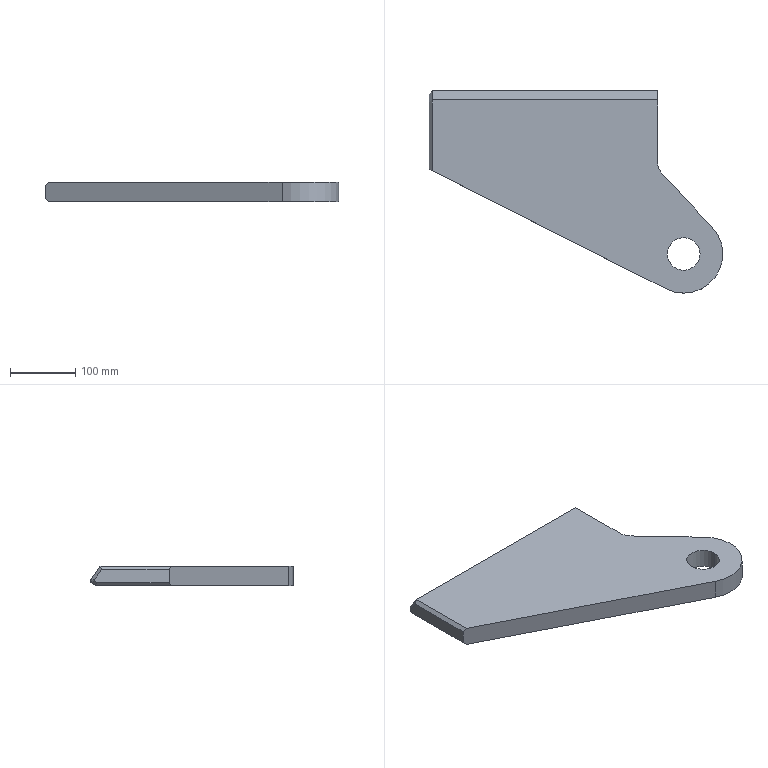Part | SolidWorks | features ICE 2, Chamfer 1, Extrusion 1, Fillet 1 | 1 solid | 18 faces | box 450 x 310 x 30 mm | volume 2452463 mm3 | plane 14 | cylinder 4 | commonest cylinder face diameters 50 x2 60 x1 120 x1
STEP:
#1=CARTESIAN_POINT('',(-25.,0.,30.));
#2=VERTEX_POINT('',#1);
#3=CARTESIAN_POINT('',(25.,0.,30.));
#4=VERTEX_POINT('',#3);
#5=CARTESIAN_POINT('',(0.,0.,30.));
#6=DIRECTION('',(0.,0.,1.));
#7=DIRECTION('',(1.,0.,0.));
#8=AXIS2_PLACEMENT_3D('',#5,#6,#7);
#9=CIRCLE('',#8,25.);
#10=EDGE_CURVE('',#2,#4,#9,.T.);
#11=ORIENTED_EDGE('',*,*,#10,.T.);
#12=CARTESIAN_POINT('',(25.,0.,0.));
#13=VERTEX_POINT('',#12);
#14=CARTESIAN_POINT('',(25.,0.,30.));
#15=DIRECTION('',(0.,0.,-1.));
#16=VECTOR('',#15,1000.);
#17=LINE('',#14,#16);
#18=EDGE_CURVE('',#4,#13,#17,.T.);
#19=ORIENTED_EDGE('',*,*,#18,.T.);
#20=CARTESIAN_POINT('',(-25.,0.,0.));
#21=VERTEX_POINT('',#20);
#22=CARTESIAN_POINT('',(0.,0.,0.));
#23=DIRECTION('',(0.,0.,1.));
#24=DIRECTION('',(1.,0.,0.));
#25=AXIS2_PLACEMENT_3D('',#22,#23,#24);
#26=CIRCLE('',#25,25.);
#27=EDGE_CURVE('',#21,#13,#26,.T.);
#28=ORIENTED_EDGE('',*,*,#27,.F.);
#29=CARTESIAN_POINT('',(-25.,0.,30.));
#30=DIRECTION('',(0.,0.,-1.));
#31=VECTOR('',#30,1000.);
#32=LINE('',#29,#31);
#33=EDGE_CURVE('',#2,#21,#32,.T.);
#34=ORIENTED_EDGE('',*,*,#33,.F.);
#35=EDGE_LOOP('',(#11,#19,#28,#34));
#36=FACE_OUTER_BOUND('',#35,.T.);
#37=CARTESIAN_POINT('',(0.,0.,30.));
#38=DIRECTION('',(0.,0.,-1.));
#39=DIRECTION('',(-1.,0.,0.));
#40=AXIS2_PLACEMENT_3D('',#37,#38,#39);
#41=CYLINDRICAL_SURFACE('',#40,25.);
#42=ADVANCED_FACE('',(#36),#41,.F.);
#43=CARTESIAN_POINT('',(-385.,235.996,30.));
#44=VERTEX_POINT('',#43);
#45=CARTESIAN_POINT('',(-40.,235.996,30.));
#46=VERTEX_POINT('',#45);
#47=CARTESIAN_POINT('',(-390.,235.996,30.));
#48=DIRECTION('',(1.,0.,0.));
#49=VECTOR('',#48,1000.);
#50=LINE('',#47,#49);
#51=EDGE_CURVE('',#44,#46,#50,.T.);
#52=ORIENTED_EDGE('',*,*,#51,.F.);
#53=CARTESIAN_POINT('',(-385.,127.471,30.));
#54=VERTEX_POINT('',#53);
#55=CARTESIAN_POINT('',(-385.,130.,30.));
#56=DIRECTION('',(0.,-1.,0.));
#57=VECTOR('',#56,1000.);
#58=LINE('',#55,#57);
#59=EDGE_CURVE('',#44,#54,#58,.T.);
#60=ORIENTED_EDGE('',*,*,#59,.T.);
#61=CARTESIAN_POINT('',(-27.078,-53.542,30.));
#62=VERTEX_POINT('',#61);
#63=CARTESIAN_POINT('',(-390.,130.,30.));
#64=DIRECTION('',(0.8924,-0.4513,0.));
#65=VECTOR('',#64,1000.);
#66=LINE('',#63,#65);
#67=EDGE_CURVE('',#54,#62,#66,.T.);
#68=ORIENTED_EDGE('',*,*,#67,.T.);
#69=CARTESIAN_POINT('',(43.682,41.133,30.));
#70=VERTEX_POINT('',#69);
#71=CARTESIAN_POINT('',(0.,0.,30.));
#72=DIRECTION('',(0.,0.,1.));
#73=DIRECTION('',(1.,0.,0.));
#74=AXIS2_PLACEMENT_3D('',#71,#72,#73);
#75=CIRCLE('',#74,60.);
#76=EDGE_CURVE('',#62,#70,#75,.T.);
#77=ORIENTED_EDGE('',*,*,#76,.T.);
#78=CARTESIAN_POINT('',(-31.841,121.335,30.));
#79=VERTEX_POINT('',#78);
#80=CARTESIAN_POINT('',(-40.,130.,30.));
#81=DIRECTION('',(-0.6855,0.728,0.));
#82=VECTOR('',#81,1000.);
#83=LINE('',#80,#82);
#84=EDGE_CURVE('',#70,#79,#83,.T.);
#85=ORIENTED_EDGE('',*,*,#84,.T.);
#86=CARTESIAN_POINT('',(-40.,141.902,30.));
#87=VERTEX_POINT('',#86);
#88=CARTESIAN_POINT('',(-10.,141.902,30.));
#89=DIRECTION('',(0.,0.,-1.));
#90=DIRECTION('',(1.,0.,0.));
#91=AXIS2_PLACEMENT_3D('',#88,#89,#90);
#92=CIRCLE('',#91,30.);
#93=EDGE_CURVE('',#79,#87,#92,.T.);
#94=ORIENTED_EDGE('',*,*,#93,.T.);
#95=CARTESIAN_POINT('',(-40.,250.,30.));
#96=DIRECTION('',(0.,1.,0.));
#97=VECTOR('',#96,1000.);
#98=LINE('',#95,#97);
#99=EDGE_CURVE('',#87,#46,#98,.T.);
#100=ORIENTED_EDGE('',*,*,#99,.T.);
#101=EDGE_LOOP('',(#52,#60,#68,#77,#85,#94,#100));
#102=FACE_OUTER_BOUND('',#101,.T.);
#103=ORIENTED_EDGE('',*,*,#10,.F.);
#104=CARTESIAN_POINT('',(0.,0.,30.));
#105=DIRECTION('',(0.,0.,1.));
#106=DIRECTION('',(1.,0.,0.));
#107=AXIS2_PLACEMENT_3D('',#104,#105,#106);
#108=CIRCLE('',#107,25.);
#109=EDGE_CURVE('',#4,#2,#108,.T.);
#110=ORIENTED_EDGE('',*,*,#109,.F.);
#111=EDGE_LOOP('',(#103,#110));
#112=FACE_BOUND('',#111,.T.);
#113=CARTESIAN_POINT('',(0.,0.,30.));
#114=DIRECTION('',(0.,0.,1.));
#115=DIRECTION('',(1.,0.,0.));
#116=AXIS2_PLACEMENT_3D('',#113,#114,#115);
#117=PLANE('',#116);
#118=ADVANCED_FACE('',(#102,#112),#117,.T.);
#119=CARTESIAN_POINT('',(-385.,127.471,0.));
#120=VERTEX_POINT('',#119);
#121=CARTESIAN_POINT('',(-27.078,-53.542,0.));
#122=VERTEX_POINT('',#121);
#123=CARTESIAN_POINT('',(-390.,130.,0.));
#124=DIRECTION('',(0.8924,-0.4513,0.));
#125=VECTOR('',#124,1000.);
#126=LINE('',#123,#125);
#127=EDGE_CURVE('',#120,#122,#126,.T.);
#128=ORIENTED_EDGE('',*,*,#127,.F.);
#129=CARTESIAN_POINT('',(-385.,242.859,0.));
#130=VERTEX_POINT('',#129);
#131=CARTESIAN_POINT('',(-385.,0.,0.));
#132=DIRECTION('',(0.,1.,0.));
#133=VECTOR('',#132,1000.);
#134=LINE('',#131,#133);
#135=EDGE_CURVE('',#120,#130,#134,.T.);
#136=ORIENTED_EDGE('',*,*,#135,.T.);
#137=CARTESIAN_POINT('',(-40.,242.859,0.));
#138=VERTEX_POINT('',#137);
#139=CARTESIAN_POINT('',(-390.,242.859,0.));
#140=DIRECTION('',(1.,0.,0.));
#141=VECTOR('',#140,1000.);
#142=LINE('',#139,#141);
#143=EDGE_CURVE('',#130,#138,#142,.T.);
#144=ORIENTED_EDGE('',*,*,#143,.T.);
#145=CARTESIAN_POINT('',(-40.,141.902,0.));
#146=VERTEX_POINT('',#145);
#147=CARTESIAN_POINT('',(-40.,250.,0.));
#148=DIRECTION('',(0.,1.,0.));
#149=VECTOR('',#148,1000.);
#150=LINE('',#147,#149);
#151=EDGE_CURVE('',#146,#138,#150,.T.);
#152=ORIENTED_EDGE('',*,*,#151,.F.);
#153=CARTESIAN_POINT('',(-31.841,121.335,0.));
#154=VERTEX_POINT('',#153);
#155=CARTESIAN_POINT('',(-10.,141.902,0.));
#156=DIRECTION('',(0.,0.,1.));
#157=DIRECTION('',(1.,0.,0.));
#158=AXIS2_PLACEMENT_3D('',#155,#156,#157);
#159=CIRCLE('',#158,30.);
#160=EDGE_CURVE('',#146,#154,#159,.T.);
#161=ORIENTED_EDGE('',*,*,#160,.T.);
#162=CARTESIAN_POINT('',(43.682,41.133,0.));
#163=VERTEX_POINT('',#162);
#164=CARTESIAN_POINT('',(-40.,130.,0.));
#165=DIRECTION('',(-0.6855,0.728,0.));
#166=VECTOR('',#165,1000.);
#167=LINE('',#164,#166);
#168=EDGE_CURVE('',#163,#154,#167,.T.);
#169=ORIENTED_EDGE('',*,*,#168,.F.);
#170=CARTESIAN_POINT('',(0.,0.,0.));
#171=DIRECTION('',(0.,0.,1.));
#172=DIRECTION('',(1.,0.,0.));
#173=AXIS2_PLACEMENT_3D('',#170,#171,#172);
#174=CIRCLE('',#173,60.);
#175=EDGE_CURVE('',#122,#163,#174,.T.);
#176=ORIENTED_EDGE('',*,*,#175,.F.);
#177=EDGE_LOOP('',(#128,#136,#144,#152,#161,#169,#176));
#178=FACE_OUTER_BOUND('',#177,.T.);
#179=ORIENTED_EDGE('',*,*,#27,.T.);
#180=CARTESIAN_POINT('',(0.,0.,0.));
#181=DIRECTION('',(0.,0.,1.));
#182=DIRECTION('',(1.,0.,0.));
#183=AXIS2_PLACEMENT_3D('',#180,#181,#182);
#184=CIRCLE('',#183,25.);
#185=EDGE_CURVE('',#13,#21,#184,.T.);
#186=ORIENTED_EDGE('',*,*,#185,.T.);
#187=EDGE_LOOP('',(#179,#186));
#188=FACE_BOUND('',#187,.T.);
#189=CARTESIAN_POINT('',(0.,0.,0.));
#190=DIRECTION('',(0.,0.,1.));
#191=DIRECTION('',(1.,0.,0.));
#192=AXIS2_PLACEMENT_3D('',#189,#190,#191);
#193=PLANE('',#192);
#194=ADVANCED_FACE('',(#178,#188),#193,.F.);
#195=ORIENTED_EDGE('',*,*,#99,.F.);
#196=CARTESIAN_POINT('',(-40.,141.902,0.));
#197=DIRECTION('',(0.,0.,-1.));
#198=VECTOR('',#197,1000.);
#199=LINE('',#196,#198);
#200=EDGE_CURVE('',#87,#146,#199,.T.);
#201=ORIENTED_EDGE('',*,*,#200,.T.);
#202=ORIENTED_EDGE('',*,*,#151,.T.);
#203=CARTESIAN_POINT('',(-40.,250.,5.));
#204=VERTEX_POINT('',#203);
#205=CARTESIAN_POINT('',(-40.,261.746,13.225));
#206=DIRECTION('',(0.,0.8192,0.5736));
#207=VECTOR('',#206,1000.);
#208=LINE('',#205,#207);
#209=EDGE_CURVE('',#138,#204,#208,.T.);
#210=ORIENTED_EDGE('',*,*,#209,.T.);
#211=CARTESIAN_POINT('',(-40.,250.,10.));
#212=VERTEX_POINT('',#211);
#213=CARTESIAN_POINT('',(-40.,250.,30.));
#214=DIRECTION('',(0.,0.,-1.));
#215=VECTOR('',#214,1000.);
#216=LINE('',#213,#215);
#217=EDGE_CURVE('',#212,#204,#216,.T.);
#218=ORIENTED_EDGE('',*,*,#217,.F.);
#219=CARTESIAN_POINT('',(-40.,240.603,23.42));
#220=DIRECTION('',(0.,-0.5736,0.8192));
#221=VECTOR('',#220,1000.);
#222=LINE('',#219,#221);
#223=EDGE_CURVE('',#212,#46,#222,.T.);
#224=ORIENTED_EDGE('',*,*,#223,.T.);
#225=EDGE_LOOP('',(#195,#201,#202,#210,#218,#224));
#226=FACE_OUTER_BOUND('',#225,.T.);
#227=CARTESIAN_POINT('',(-40.,250.,30.));
#228=DIRECTION('',(-1.,0.,0.));
#229=DIRECTION('',(0.,0.,1.));
#230=AXIS2_PLACEMENT_3D('',#227,#228,#229);
#231=PLANE('',#230);
#232=ADVANCED_FACE('',(#226),#231,.F.);
#233=CARTESIAN_POINT('',(-385.,250.,5.));
#234=VERTEX_POINT('',#233);
#235=CARTESIAN_POINT('',(-390.,250.,5.));
#236=DIRECTION('',(1.,0.,0.));
#237=VECTOR('',#236,1000.);
#238=LINE('',#235,#237);
#239=EDGE_CURVE('',#234,#204,#238,.T.);
#240=ORIENTED_EDGE('',*,*,#239,.F.);
#241=CARTESIAN_POINT('',(-385.,250.,10.));
#242=VERTEX_POINT('',#241);
#243=CARTESIAN_POINT('',(-385.,250.,30.));
#244=DIRECTION('',(0.,0.,1.));
#245=VECTOR('',#244,1000.);
#246=LINE('',#243,#245);
#247=EDGE_CURVE('',#234,#242,#246,.T.);
#248=ORIENTED_EDGE('',*,*,#247,.T.);
#249=CARTESIAN_POINT('',(-390.,250.,10.));
#250=DIRECTION('',(1.,0.,0.));
#251=VECTOR('',#250,1000.);
#252=LINE('',#249,#251);
#253=EDGE_CURVE('',#242,#212,#252,.T.);
#254=ORIENTED_EDGE('',*,*,#253,.T.);
#255=ORIENTED_EDGE('',*,*,#217,.T.);
#256=EDGE_LOOP('',(#240,#248,#254,#255));
#257=FACE_OUTER_BOUND('',#256,.T.);
#258=CARTESIAN_POINT('',(-40.,250.,30.));
#259=DIRECTION('',(0.,-1.,0.));
#260=DIRECTION('',(1.,0.,0.));
#261=AXIS2_PLACEMENT_3D('',#258,#259,#260);
#262=PLANE('',#261);
#263=ADVANCED_FACE('',(#257),#262,.F.);
#264=CARTESIAN_POINT('',(-390.,130.,25.));
#265=VERTEX_POINT('',#264);
#266=CARTESIAN_POINT('',(-390.,130.,5.));
#267=VERTEX_POINT('',#266);
#268=CARTESIAN_POINT('',(-390.,130.,30.));
#269=DIRECTION('',(0.,0.,-1.));
#270=VECTOR('',#269,1000.);
#271=LINE('',#268,#270);
#272=EDGE_CURVE('',#265,#267,#271,.T.);
#273=ORIENTED_EDGE('',*,*,#272,.F.);
#274=CARTESIAN_POINT('',(-390.,233.393,25.));
#275=VERTEX_POINT('',#274);
#276=CARTESIAN_POINT('',(-390.,235.996,25.));
#277=DIRECTION('',(0.,1.,0.));
#278=VECTOR('',#277,1000.);
#279=LINE('',#276,#278);
#280=EDGE_CURVE('',#265,#275,#279,.T.);
#281=ORIENTED_EDGE('',*,*,#280,.T.);
#282=CARTESIAN_POINT('',(-390.,245.,8.424));
#283=VERTEX_POINT('',#282);
#284=CARTESIAN_POINT('',(-390.,236.507,20.552));
#285=DIRECTION('',(0.,0.5736,-0.8192));
#286=VECTOR('',#285,1000.);
#287=LINE('',#284,#286);
#288=EDGE_CURVE('',#275,#283,#287,.T.);
#289=ORIENTED_EDGE('',*,*,#288,.T.);
#290=CARTESIAN_POINT('',(-390.,245.,7.603));
#291=VERTEX_POINT('',#290);
#292=CARTESIAN_POINT('',(-390.,245.,30.));
#293=DIRECTION('',(0.,0.,-1.));
#294=VECTOR('',#293,1000.);
#295=LINE('',#292,#294);
#296=EDGE_CURVE('',#283,#291,#295,.T.);
#297=ORIENTED_EDGE('',*,*,#296,.T.);
#298=CARTESIAN_POINT('',(-390.,241.283,5.));
#299=VERTEX_POINT('',#298);
#300=CARTESIAN_POINT('',(-390.,258.878,17.321));
#301=DIRECTION('',(0.,-0.8192,-0.5736));
#302=VECTOR('',#301,1000.);
#303=LINE('',#300,#302);
#304=EDGE_CURVE('',#291,#299,#303,.T.);
#305=ORIENTED_EDGE('',*,*,#304,.T.);
#306=CARTESIAN_POINT('',(-390.,250.,5.));
#307=DIRECTION('',(0.,-1.,0.));
#308=VECTOR('',#307,1000.);
#309=LINE('',#306,#308);
#310=EDGE_CURVE('',#299,#267,#309,.T.);
#311=ORIENTED_EDGE('',*,*,#310,.T.);
#312=EDGE_LOOP('',(#273,#281,#289,#297,#305,#311));
#313=FACE_OUTER_BOUND('',#312,.T.);
#314=CARTESIAN_POINT('',(-390.,250.,30.));
#315=DIRECTION('',(1.,0.,0.));
#316=DIRECTION('',(0.,1.,0.));
#317=AXIS2_PLACEMENT_3D('',#314,#315,#316);
#318=PLANE('',#317);
#319=ADVANCED_FACE('',(#313),#318,.F.);
#320=ORIENTED_EDGE('',*,*,#67,.F.);
#321=CARTESIAN_POINT('',(-356.421,113.018,58.579));
#322=DIRECTION('',(-0.6658,0.3367,-0.6658));
#323=VECTOR('',#322,1000.);
#324=LINE('',#321,#323);
#325=EDGE_CURVE('',#54,#265,#324,.T.);
#326=ORIENTED_EDGE('',*,*,#325,.T.);
#327=ORIENTED_EDGE('',*,*,#272,.T.);
#328=CARTESIAN_POINT('',(-416.904,143.606,31.904));
#329=DIRECTION('',(0.6658,-0.3367,-0.6658));
#330=VECTOR('',#329,1000.);
#331=LINE('',#328,#330);
#332=EDGE_CURVE('',#267,#120,#331,.T.);
#333=ORIENTED_EDGE('',*,*,#332,.T.);
#334=ORIENTED_EDGE('',*,*,#127,.T.);
#335=CARTESIAN_POINT('',(-27.078,-53.542,30.));
#336=DIRECTION('',(0.,0.,-1.));
#337=VECTOR('',#336,1000.);
#338=LINE('',#335,#337);
#339=EDGE_CURVE('',#62,#122,#338,.T.);
#340=ORIENTED_EDGE('',*,*,#339,.F.);
#341=EDGE_LOOP('',(#320,#326,#327,#333,#334,#340));
#342=FACE_OUTER_BOUND('',#341,.T.);
#343=CARTESIAN_POINT('',(-390.,130.,30.));
#344=DIRECTION('',(0.4513,0.8924,0.));
#345=DIRECTION('',(-0.8924,0.4513,0.));
#346=AXIS2_PLACEMENT_3D('',#343,#344,#345);
#347=PLANE('',#346);
#348=ADVANCED_FACE('',(#342),#347,.F.);
#349=ORIENTED_EDGE('',*,*,#175,.T.);
#350=CARTESIAN_POINT('',(43.682,41.133,30.));
#351=DIRECTION('',(0.,0.,-1.));
#352=VECTOR('',#351,1000.);
#353=LINE('',#350,#352);
#354=EDGE_CURVE('',#70,#163,#353,.T.);
#355=ORIENTED_EDGE('',*,*,#354,.F.);
#356=ORIENTED_EDGE('',*,*,#76,.F.);
#357=ORIENTED_EDGE('',*,*,#339,.T.);
#358=EDGE_LOOP('',(#349,#355,#356,#357));
#359=FACE_OUTER_BOUND('',#358,.T.);
#360=CARTESIAN_POINT('',(0.,0.,30.));
#361=DIRECTION('',(0.,0.,-1.));
#362=DIRECTION('',(-1.,0.,0.));
#363=AXIS2_PLACEMENT_3D('',#360,#361,#362);
#364=CYLINDRICAL_SURFACE('',#363,60.);
#365=ADVANCED_FACE('',(#359),#364,.T.);
#366=ORIENTED_EDGE('',*,*,#168,.T.);
#367=CARTESIAN_POINT('',(-31.841,121.335,30.));
#368=DIRECTION('',(0.,0.,1.));
#369=VECTOR('',#368,1000.);
#370=LINE('',#367,#369);
#371=EDGE_CURVE('',#154,#79,#370,.T.);
#372=ORIENTED_EDGE('',*,*,#371,.T.);
#373=ORIENTED_EDGE('',*,*,#84,.F.);
#374=ORIENTED_EDGE('',*,*,#354,.T.);
#375=EDGE_LOOP('',(#366,#372,#373,#374));
#376=FACE_OUTER_BOUND('',#375,.T.);
#377=CARTESIAN_POINT('',(-40.,130.,30.));
#378=DIRECTION('',(-0.728,-0.6855,0.));
#379=DIRECTION('',(0.6855,-0.728,0.));
#380=AXIS2_PLACEMENT_3D('',#377,#378,#379);
#381=PLANE('',#380);
#382=ADVANCED_FACE('',(#376),#381,.F.);
#383=ORIENTED_EDGE('',*,*,#18,.F.);
#384=ORIENTED_EDGE('',*,*,#109,.T.);
#385=ORIENTED_EDGE('',*,*,#33,.T.);
#386=ORIENTED_EDGE('',*,*,#185,.F.);
#387=EDGE_LOOP('',(#383,#384,#385,#386));
#388=FACE_OUTER_BOUND('',#387,.T.);
#389=CARTESIAN_POINT('',(0.,0.,30.));
#390=DIRECTION('',(0.,0.,-1.));
#391=DIRECTION('',(-1.,0.,0.));
#392=AXIS2_PLACEMENT_3D('',#389,#390,#391);
#393=CYLINDRICAL_SURFACE('',#392,25.);
#394=ADVANCED_FACE('',(#388),#393,.F.);
#395=ORIENTED_EDGE('',*,*,#253,.F.);
#396=CARTESIAN_POINT('',(-385.,250.,10.));
#397=DIRECTION('',(0.,-0.5736,0.8192));
#398=VECTOR('',#397,1000.);
#399=LINE('',#396,#398);
#400=EDGE_CURVE('',#242,#44,#399,.T.);
#401=ORIENTED_EDGE('',*,*,#400,.T.);
#402=ORIENTED_EDGE('',*,*,#51,.T.);
#403=ORIENTED_EDGE('',*,*,#223,.F.);
#404=EDGE_LOOP('',(#395,#401,#402,#403));
#405=FACE_OUTER_BOUND('',#404,.T.);
#406=CARTESIAN_POINT('',(-390.,250.,10.));
#407=DIRECTION('',(0.,-0.8192,-0.5736));
#408=DIRECTION('',(0.,0.5736,-0.8192));
#409=AXIS2_PLACEMENT_3D('',#406,#407,#408);
#410=PLANE('',#409);
#411=ADVANCED_FACE('',(#405),#410,.F.);
#412=ORIENTED_EDGE('',*,*,#143,.F.);
#413=CARTESIAN_POINT('',(-385.,250.,5.));
#414=DIRECTION('',(0.,0.8192,0.5736));
#415=VECTOR('',#414,1000.);
#416=LINE('',#413,#415);
#417=EDGE_CURVE('',#130,#234,#416,.T.);
#418=ORIENTED_EDGE('',*,*,#417,.T.);
#419=ORIENTED_EDGE('',*,*,#239,.T.);
#420=ORIENTED_EDGE('',*,*,#209,.F.);
#421=EDGE_LOOP('',(#412,#418,#419,#420));
#422=FACE_OUTER_BOUND('',#421,.T.);
#423=CARTESIAN_POINT('',(-390.,250.,5.));
#424=DIRECTION('',(0.,-0.5736,0.8192));
#425=DIRECTION('',(0.,-0.8192,-0.5736));
#426=AXIS2_PLACEMENT_3D('',#423,#424,#425);
#427=PLANE('',#426);
#428=ADVANCED_FACE('',(#422),#427,.F.);
#429=ORIENTED_EDGE('',*,*,#332,.F.);
#430=ORIENTED_EDGE('',*,*,#310,.F.);
#431=CARTESIAN_POINT('',(-388.691,241.696,3.691));
#432=DIRECTION('',(-0.6902,-0.2176,0.6902));
#433=VECTOR('',#432,1000.);
#434=LINE('',#431,#433);
#435=EDGE_CURVE('',#130,#299,#434,.T.);
#436=ORIENTED_EDGE('',*,*,#435,.F.);
#437=ORIENTED_EDGE('',*,*,#135,.F.);
#438=EDGE_LOOP('',(#429,#430,#436,#437));
#439=FACE_OUTER_BOUND('',#438,.T.);
#440=CARTESIAN_POINT('',(-390.,250.,5.));
#441=DIRECTION('',(0.7071,0.,0.7071));
#442=DIRECTION('',(0.,-1.,0.));
#443=AXIS2_PLACEMENT_3D('',#440,#441,#442);
#444=PLANE('',#443);
#445=ADVANCED_FACE('',(#439),#444,.F.);
#446=ORIENTED_EDGE('',*,*,#435,.T.);
#447=ORIENTED_EDGE('',*,*,#304,.F.);
#448=CARTESIAN_POINT('',(-386.116,248.884,5.581));
#449=DIRECTION('',(-0.6636,-0.6636,0.3454));
#450=VECTOR('',#449,1000.);
#451=LINE('',#448,#450);
#452=EDGE_CURVE('',#234,#291,#451,.T.);
#453=ORIENTED_EDGE('',*,*,#452,.F.);
#454=ORIENTED_EDGE('',*,*,#417,.F.);
#455=EDGE_LOOP('',(#446,#447,#453,#454));
#456=FACE_OUTER_BOUND('',#455,.T.);
#457=CARTESIAN_POINT('',(-390.,258.878,17.321));
#458=DIRECTION('',(0.7071,-0.4056,0.5792));
#459=DIRECTION('',(0.,-0.8192,-0.5736));
#460=AXIS2_PLACEMENT_3D('',#457,#458,#459);
#461=PLANE('',#460);
#462=ADVANCED_FACE('',(#456),#461,.F.);
#463=ORIENTED_EDGE('',*,*,#452,.T.);
#464=ORIENTED_EDGE('',*,*,#296,.F.);
#465=CARTESIAN_POINT('',(-386.76,248.24,9.445));
#466=DIRECTION('',(-0.6902,-0.6902,-0.2176));
#467=VECTOR('',#466,1000.);
#468=LINE('',#465,#467);
#469=EDGE_CURVE('',#242,#283,#468,.T.);
#470=ORIENTED_EDGE('',*,*,#469,.F.);
#471=ORIENTED_EDGE('',*,*,#247,.F.);
#472=EDGE_LOOP('',(#463,#464,#470,#471));
#473=FACE_OUTER_BOUND('',#472,.T.);
#474=CARTESIAN_POINT('',(-390.,245.,30.));
#475=DIRECTION('',(0.7071,-0.7071,0.));
#476=DIRECTION('',(0.,0.,-1.));
#477=AXIS2_PLACEMENT_3D('',#474,#475,#476);
#478=PLANE('',#477);
#479=ADVANCED_FACE('',(#473),#478,.F.);
#480=ORIENTED_EDGE('',*,*,#469,.T.);
#481=ORIENTED_EDGE('',*,*,#288,.F.);
#482=CARTESIAN_POINT('',(-391.245,232.745,23.755));
#483=DIRECTION('',(-0.6636,-0.3454,-0.6636));
#484=VECTOR('',#483,1000.);
#485=LINE('',#482,#484);
#486=EDGE_CURVE('',#44,#275,#485,.T.);
#487=ORIENTED_EDGE('',*,*,#486,.F.);
#488=ORIENTED_EDGE('',*,*,#400,.F.);
#489=EDGE_LOOP('',(#480,#481,#487,#488));
#490=FACE_OUTER_BOUND('',#489,.T.);
#491=CARTESIAN_POINT('',(-390.,236.507,20.552));
#492=DIRECTION('',(0.7071,-0.5792,-0.4056));
#493=DIRECTION('',(0.,0.5736,-0.8192));
#494=AXIS2_PLACEMENT_3D('',#491,#492,#493);
#495=PLANE('',#494);
#496=ADVANCED_FACE('',(#490),#495,.F.);
#497=ORIENTED_EDGE('',*,*,#486,.T.);
#498=ORIENTED_EDGE('',*,*,#280,.F.);
#499=ORIENTED_EDGE('',*,*,#325,.F.);
#500=ORIENTED_EDGE('',*,*,#59,.F.);
#501=EDGE_LOOP('',(#497,#498,#499,#500));
#502=FACE_OUTER_BOUND('',#501,.T.);
#503=CARTESIAN_POINT('',(-385.,0.,30.));
#504=DIRECTION('',(-0.7071,0.,0.7071));
#505=DIRECTION('',(0.,1.,0.));
#506=AXIS2_PLACEMENT_3D('',#503,#504,#505);
#507=PLANE('',#506);
#508=ADVANCED_FACE('',(#502),#507,.T.);
#509=ORIENTED_EDGE('',*,*,#93,.F.);
#510=ORIENTED_EDGE('',*,*,#371,.F.);
#511=ORIENTED_EDGE('',*,*,#160,.F.);
#512=ORIENTED_EDGE('',*,*,#200,.F.);
#513=EDGE_LOOP('',(#509,#510,#511,#512));
#514=FACE_OUTER_BOUND('',#513,.T.);
#515=CARTESIAN_POINT('',(-10.,141.902,30.));
#516=DIRECTION('',(0.,0.,1.));
#517=DIRECTION('',(1.,0.,0.));
#518=AXIS2_PLACEMENT_3D('',#515,#516,#517);
#519=CYLINDRICAL_SURFACE('',#518,30.);
#520=ADVANCED_FACE('',(#514),#519,.F.);
#521=CLOSED_SHELL('',(#42,#118,#194,#232,#263,#319,#348,#365,#382,#394,#411,#428,#445,#462,#479,#496,#508,#520));
#522=MANIFOLD_SOLID_BREP('',#521);
#523=CARTESIAN_POINT('',(0.,0.,0.));
#524=DIRECTION('',(0.,0.,1.));
#525=DIRECTION('',(1.,0.,0.));
#526=AXIS2_PLACEMENT_3D('',#523,#524,#525);
#527=(LENGTH_UNIT()NAMED_UNIT(*)SI_UNIT(.MILLI.,.METRE.));
#528=UNCERTAINTY_MEASURE_WITH_UNIT(LENGTH_MEASURE(0.00001),#527,'','');
#529=(NAMED_UNIT(*)PLANE_ANGLE_UNIT()SI_UNIT($,.RADIAN.));
#530=(NAMED_UNIT(*)SI_UNIT($,.STERADIAN.)SOLID_ANGLE_UNIT());
#531=(GEOMETRIC_REPRESENTATION_CONTEXT(3)GLOBAL_UNCERTAINTY_ASSIGNED_CONTEXT((#528))GLOBAL_UNIT_ASSIGNED_CONTEXT((#527,#529,#530))REPRESENTATION_CONTEXT('',''));
#532=ADVANCED_BREP_SHAPE_REPRESENTATION('',(#522,#526),#531);